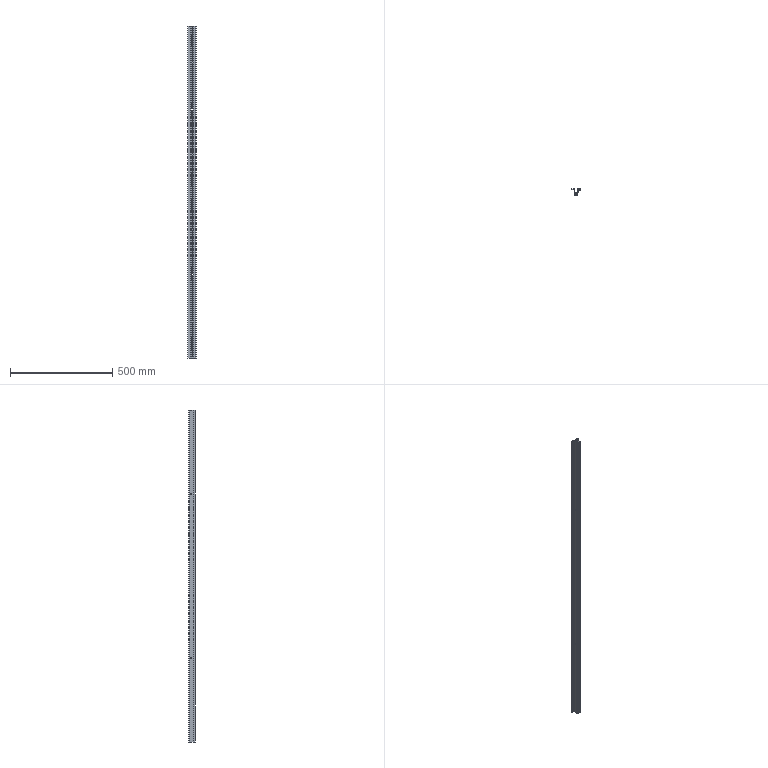Part | 1 solid | 102 faces | box 40 x 29.5 x 1620 mm | volume 304588 mm3 | plane 65 | cylinder 37 | commonest cylinder face diameters 9 x30 2 x5 3 x2